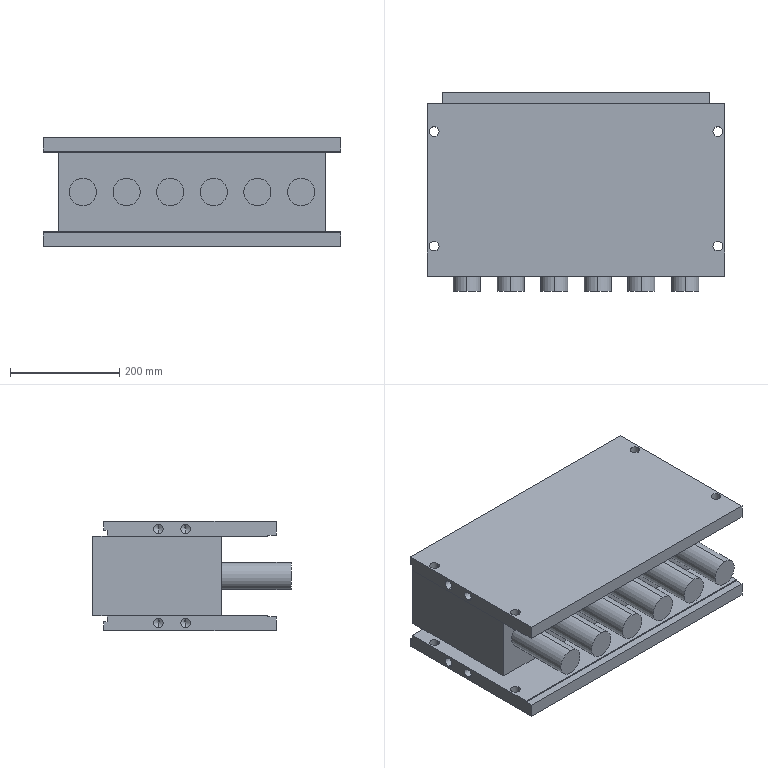Part | STEP file | mold 06_default | 1 solid | 134 faces | box 545 x 363.5 x 200 mm | volume 24295662 mm3 | cylinder 68 | plane 38 | cone 16 | spline 12 | commonest cylinder face diameters 17.5 x16 18 x16 24 x12 50 x12 65 x12